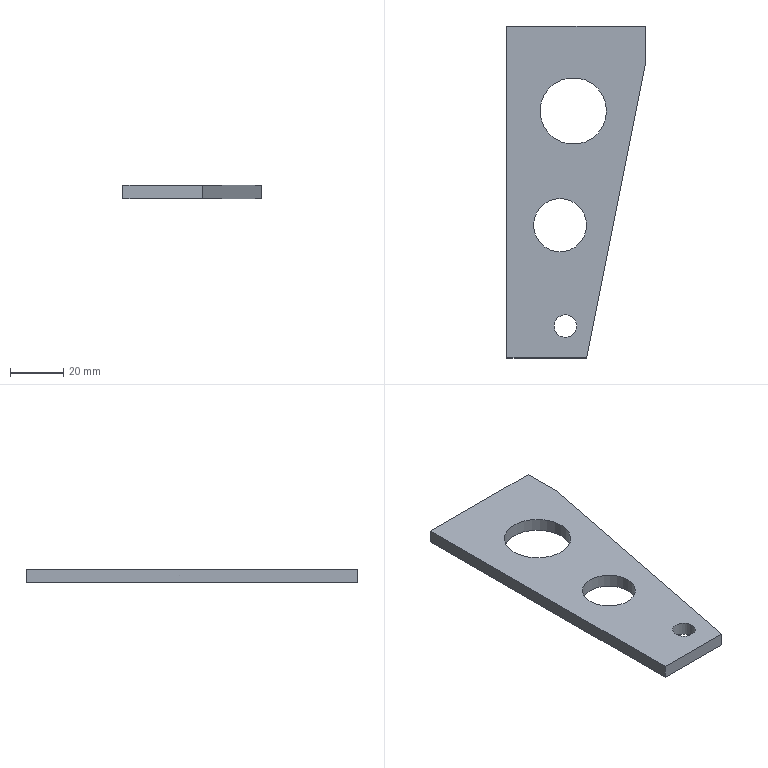Part | NX | features DATUM_CSYS 1, EXTRACT_DATUM_PLANE 1, EXTRUDE 1, SKETCH 1 | 1 solid | 10 faces | box 52 x 125 x 5 mm | volume 22141 mm3 | plane 7 | cylinder 3 | commonest cylinder face diameters 8.5 x1 20 x1 25 x1
STEP:
#1=CARTESIAN_POINT('',(-32.5,32.5,2.5));
#2=VERTEX_POINT('',#1);
#3=CARTESIAN_POINT('',(-32.5,-92.5,2.5));
#4=VERTEX_POINT('',#3);
#5=CARTESIAN_POINT('',(-32.5,32.5,2.5));
#6=DIRECTION('',(0.,-1.,0.));
#7=VECTOR('',#6,1000.);
#8=LINE('',#5,#7);
#9=EDGE_CURVE('',#2,#4,#8,.T.);
#10=ORIENTED_EDGE('',*,*,#9,.F.);
#11=CARTESIAN_POINT('',(-32.5,32.5,-2.5));
#12=VERTEX_POINT('',#11);
#13=CARTESIAN_POINT('',(-32.5,32.5,-2.5));
#14=DIRECTION('',(0.,0.,1.));
#15=VECTOR('',#14,1000.);
#16=LINE('',#13,#15);
#17=EDGE_CURVE('',#12,#2,#16,.T.);
#18=ORIENTED_EDGE('',*,*,#17,.F.);
#19=CARTESIAN_POINT('',(-32.5,-92.5,-2.5));
#20=VERTEX_POINT('',#19);
#21=CARTESIAN_POINT('',(-32.5,32.5,-2.5));
#22=DIRECTION('',(0.,-1.,0.));
#23=VECTOR('',#22,1000.);
#24=LINE('',#21,#23);
#25=EDGE_CURVE('',#12,#20,#24,.T.);
#26=ORIENTED_EDGE('',*,*,#25,.T.);
#27=CARTESIAN_POINT('',(-32.5,-92.5,-2.5));
#28=DIRECTION('',(0.,0.,1.));
#29=VECTOR('',#28,1000.);
#30=LINE('',#27,#29);
#31=EDGE_CURVE('',#20,#4,#30,.T.);
#32=ORIENTED_EDGE('',*,*,#31,.T.);
#33=EDGE_LOOP('',(#10,#18,#26,#32));
#34=FACE_BOUND('',#33,.T.);
#35=CARTESIAN_POINT('',(-32.5,32.5,-2.5));
#36=DIRECTION('',(-1.,0.,0.));
#37=DIRECTION('',(0.,0.,1.));
#38=AXIS2_PLACEMENT_3D('',#35,#36,#37);
#39=PLANE('',#38);
#40=ADVANCED_FACE('',(#34),#39,.T.);
#41=CARTESIAN_POINT('',(-2.5,-92.5,2.5));
#42=VERTEX_POINT('',#41);
#43=CARTESIAN_POINT('',(-32.5,-92.5,2.5));
#44=DIRECTION('',(1.,0.,0.));
#45=VECTOR('',#44,1000.);
#46=LINE('',#43,#45);
#47=EDGE_CURVE('',#4,#42,#46,.T.);
#48=ORIENTED_EDGE('',*,*,#47,.F.);
#49=ORIENTED_EDGE('',*,*,#31,.F.);
#50=CARTESIAN_POINT('',(-2.5,-92.5,-2.5));
#51=VERTEX_POINT('',#50);
#52=CARTESIAN_POINT('',(-32.5,-92.5,-2.5));
#53=DIRECTION('',(1.,0.,0.));
#54=VECTOR('',#53,1000.);
#55=LINE('',#52,#54);
#56=EDGE_CURVE('',#20,#51,#55,.T.);
#57=ORIENTED_EDGE('',*,*,#56,.T.);
#58=CARTESIAN_POINT('',(-2.5,-92.5,-2.5));
#59=DIRECTION('',(0.,0.,1.));
#60=VECTOR('',#59,1000.);
#61=LINE('',#58,#60);
#62=EDGE_CURVE('',#51,#42,#61,.T.);
#63=ORIENTED_EDGE('',*,*,#62,.T.);
#64=EDGE_LOOP('',(#48,#49,#57,#63));
#65=FACE_BOUND('',#64,.T.);
#66=CARTESIAN_POINT('',(-32.5,-92.5,-2.5));
#67=DIRECTION('',(0.,-1.,0.));
#68=DIRECTION('',(0.,0.,-1.));
#69=AXIS2_PLACEMENT_3D('',#66,#67,#68);
#70=PLANE('',#69);
#71=ADVANCED_FACE('',(#65),#70,.T.);
#72=CARTESIAN_POINT('',(19.5,17.5,2.5));
#73=VERTEX_POINT('',#72);
#74=CARTESIAN_POINT('',(-2.5,-92.5,2.5));
#75=DIRECTION('',(0.1961,0.9806,0.));
#76=VECTOR('',#75,1000.);
#77=LINE('',#74,#76);
#78=EDGE_CURVE('',#42,#73,#77,.T.);
#79=ORIENTED_EDGE('',*,*,#78,.F.);
#80=ORIENTED_EDGE('',*,*,#62,.F.);
#81=CARTESIAN_POINT('',(19.5,17.5,-2.5));
#82=VERTEX_POINT('',#81);
#83=CARTESIAN_POINT('',(-2.5,-92.5,-2.5));
#84=DIRECTION('',(0.1961,0.9806,0.));
#85=VECTOR('',#84,1000.);
#86=LINE('',#83,#85);
#87=EDGE_CURVE('',#51,#82,#86,.T.);
#88=ORIENTED_EDGE('',*,*,#87,.T.);
#89=CARTESIAN_POINT('',(19.5,17.5,-2.5));
#90=DIRECTION('',(0.,0.,1.));
#91=VECTOR('',#90,1000.);
#92=LINE('',#89,#91);
#93=EDGE_CURVE('',#82,#73,#92,.T.);
#94=ORIENTED_EDGE('',*,*,#93,.T.);
#95=EDGE_LOOP('',(#79,#80,#88,#94));
#96=FACE_BOUND('',#95,.T.);
#97=CARTESIAN_POINT('',(-2.5,-92.5,-2.5));
#98=DIRECTION('',(0.9806,-0.1961,0.));
#99=DIRECTION('',(0.1961,0.9806,0.));
#100=AXIS2_PLACEMENT_3D('',#97,#98,#99);
#101=PLANE('',#100);
#102=ADVANCED_FACE('',(#96),#101,.T.);
#103=CARTESIAN_POINT('',(19.5,32.5,2.5));
#104=VERTEX_POINT('',#103);
#105=CARTESIAN_POINT('',(19.5,17.5,2.5));
#106=DIRECTION('',(0.,1.,0.));
#107=VECTOR('',#106,1000.);
#108=LINE('',#105,#107);
#109=EDGE_CURVE('',#73,#104,#108,.T.);
#110=ORIENTED_EDGE('',*,*,#109,.F.);
#111=ORIENTED_EDGE('',*,*,#93,.F.);
#112=CARTESIAN_POINT('',(19.5,32.5,-2.5));
#113=VERTEX_POINT('',#112);
#114=CARTESIAN_POINT('',(19.5,17.5,-2.5));
#115=DIRECTION('',(0.,1.,0.));
#116=VECTOR('',#115,1000.);
#117=LINE('',#114,#116);
#118=EDGE_CURVE('',#82,#113,#117,.T.);
#119=ORIENTED_EDGE('',*,*,#118,.T.);
#120=CARTESIAN_POINT('',(19.5,32.5,-2.5));
#121=DIRECTION('',(0.,0.,1.));
#122=VECTOR('',#121,1000.);
#123=LINE('',#120,#122);
#124=EDGE_CURVE('',#113,#104,#123,.T.);
#125=ORIENTED_EDGE('',*,*,#124,.T.);
#126=EDGE_LOOP('',(#110,#111,#119,#125));
#127=FACE_BOUND('',#126,.T.);
#128=CARTESIAN_POINT('',(19.5,17.5,-2.5));
#129=DIRECTION('',(1.,0.,0.));
#130=DIRECTION('',(0.,0.,-1.));
#131=AXIS2_PLACEMENT_3D('',#128,#129,#130);
#132=PLANE('',#131);
#133=ADVANCED_FACE('',(#127),#132,.T.);
#134=CARTESIAN_POINT('',(-20.,0.5,2.5));
#135=VERTEX_POINT('',#134);
#136=CARTESIAN_POINT('',(-7.5,0.5,2.5));
#137=DIRECTION('',(0.,0.,-1.));
#138=DIRECTION('',(-1.,0.,0.));
#139=AXIS2_PLACEMENT_3D('',#136,#137,#138);
#140=CIRCLE('',#139,12.5);
#141=EDGE_CURVE('',#135,#135,#140,.T.);
#142=ORIENTED_EDGE('',*,*,#141,.F.);
#143=EDGE_LOOP('',(#142));
#144=FACE_BOUND('',#143,.T.);
#145=CARTESIAN_POINT('',(5.,0.5,-2.5));
#146=VERTEX_POINT('',#145);
#147=CARTESIAN_POINT('',(-7.5,0.5,-2.5));
#148=DIRECTION('',(0.,0.,-1.));
#149=DIRECTION('',(1.,0.,0.));
#150=AXIS2_PLACEMENT_3D('',#147,#148,#149);
#151=CIRCLE('',#150,12.5);
#152=EDGE_CURVE('',#146,#146,#151,.T.);
#153=ORIENTED_EDGE('',*,*,#152,.T.);
#154=EDGE_LOOP('',(#153));
#155=FACE_BOUND('',#154,.T.);
#156=CARTESIAN_POINT('',(-7.5,0.5,-2.5));
#157=DIRECTION('',(0.,0.,1.));
#158=DIRECTION('',(1.,0.,0.));
#159=AXIS2_PLACEMENT_3D('',#156,#157,#158);
#160=CYLINDRICAL_SURFACE('',#159,12.5);
#161=ADVANCED_FACE('',(#144,#155),#160,.F.);
#162=CARTESIAN_POINT('',(-22.5,-42.5,2.5));
#163=VERTEX_POINT('',#162);
#164=CARTESIAN_POINT('',(-12.5,-42.5,2.5));
#165=DIRECTION('',(0.,0.,-1.));
#166=DIRECTION('',(-1.,0.,0.));
#167=AXIS2_PLACEMENT_3D('',#164,#165,#166);
#168=CIRCLE('',#167,10.);
#169=EDGE_CURVE('',#163,#163,#168,.T.);
#170=ORIENTED_EDGE('',*,*,#169,.F.);
#171=EDGE_LOOP('',(#170));
#172=FACE_BOUND('',#171,.T.);
#173=CARTESIAN_POINT('',(-2.5,-42.5,-2.5));
#174=VERTEX_POINT('',#173);
#175=CARTESIAN_POINT('',(-12.5,-42.5,-2.5));
#176=DIRECTION('',(0.,0.,-1.));
#177=DIRECTION('',(1.,0.,0.));
#178=AXIS2_PLACEMENT_3D('',#175,#176,#177);
#179=CIRCLE('',#178,10.);
#180=EDGE_CURVE('',#174,#174,#179,.T.);
#181=ORIENTED_EDGE('',*,*,#180,.T.);
#182=EDGE_LOOP('',(#181));
#183=FACE_BOUND('',#182,.T.);
#184=CARTESIAN_POINT('',(-12.5,-42.5,-2.5));
#185=DIRECTION('',(0.,0.,1.));
#186=DIRECTION('',(1.,0.,0.));
#187=AXIS2_PLACEMENT_3D('',#184,#185,#186);
#188=CYLINDRICAL_SURFACE('',#187,10.);
#189=ADVANCED_FACE('',(#172,#183),#188,.F.);
#190=CARTESIAN_POINT('',(19.5,32.5,2.5));
#191=DIRECTION('',(-1.,0.,0.));
#192=VECTOR('',#191,1000.);
#193=LINE('',#190,#192);
#194=EDGE_CURVE('',#104,#2,#193,.T.);
#195=ORIENTED_EDGE('',*,*,#194,.F.);
#196=ORIENTED_EDGE('',*,*,#124,.F.);
#197=CARTESIAN_POINT('',(19.5,32.5,-2.5));
#198=DIRECTION('',(-1.,0.,0.));
#199=VECTOR('',#198,1000.);
#200=LINE('',#197,#199);
#201=EDGE_CURVE('',#113,#12,#200,.T.);
#202=ORIENTED_EDGE('',*,*,#201,.T.);
#203=ORIENTED_EDGE('',*,*,#17,.T.);
#204=EDGE_LOOP('',(#195,#196,#202,#203));
#205=FACE_BOUND('',#204,.T.);
#206=CARTESIAN_POINT('',(19.5,32.5,-2.5));
#207=DIRECTION('',(0.,1.,0.));
#208=DIRECTION('',(0.,0.,1.));
#209=AXIS2_PLACEMENT_3D('',#206,#207,#208);
#210=PLANE('',#209);
#211=ADVANCED_FACE('',(#205),#210,.T.);
#212=CARTESIAN_POINT('',(-14.75,-80.5,2.5));
#213=VERTEX_POINT('',#212);
#214=CARTESIAN_POINT('',(-10.5,-80.5,2.5));
#215=DIRECTION('',(0.,0.,-1.));
#216=DIRECTION('',(-1.,0.,0.));
#217=AXIS2_PLACEMENT_3D('',#214,#215,#216);
#218=CIRCLE('',#217,4.25);
#219=EDGE_CURVE('',#213,#213,#218,.T.);
#220=ORIENTED_EDGE('',*,*,#219,.F.);
#221=EDGE_LOOP('',(#220));
#222=FACE_BOUND('',#221,.T.);
#223=CARTESIAN_POINT('',(-6.25,-80.5,-2.5));
#224=VERTEX_POINT('',#223);
#225=CARTESIAN_POINT('',(-10.5,-80.5,-2.5));
#226=DIRECTION('',(0.,0.,-1.));
#227=DIRECTION('',(1.,0.,0.));
#228=AXIS2_PLACEMENT_3D('',#225,#226,#227);
#229=CIRCLE('',#228,4.25);
#230=EDGE_CURVE('',#224,#224,#229,.T.);
#231=ORIENTED_EDGE('',*,*,#230,.T.);
#232=EDGE_LOOP('',(#231));
#233=FACE_BOUND('',#232,.T.);
#234=CARTESIAN_POINT('',(-10.5,-80.5,-2.5));
#235=DIRECTION('',(0.,0.,1.));
#236=DIRECTION('',(1.,0.,0.));
#237=AXIS2_PLACEMENT_3D('',#234,#235,#236);
#238=CYLINDRICAL_SURFACE('',#237,4.25);
#239=ADVANCED_FACE('',(#222,#233),#238,.F.);
#240=ORIENTED_EDGE('',*,*,#25,.F.);
#241=ORIENTED_EDGE('',*,*,#201,.F.);
#242=ORIENTED_EDGE('',*,*,#118,.F.);
#243=ORIENTED_EDGE('',*,*,#87,.F.);
#244=ORIENTED_EDGE('',*,*,#56,.F.);
#245=EDGE_LOOP('',(#240,#241,#242,#243,#244));
#246=FACE_BOUND('',#245,.T.);
#247=ORIENTED_EDGE('',*,*,#180,.F.);
#248=EDGE_LOOP('',(#247));
#249=FACE_BOUND('',#248,.T.);
#250=ORIENTED_EDGE('',*,*,#152,.F.);
#251=EDGE_LOOP('',(#250));
#252=FACE_BOUND('',#251,.T.);
#253=ORIENTED_EDGE('',*,*,#230,.F.);
#254=EDGE_LOOP('',(#253));
#255=FACE_BOUND('',#254,.T.);
#256=CARTESIAN_POINT('',(-12.5,-42.5,-2.5));
#257=DIRECTION('',(0.,0.,-1.));
#258=DIRECTION('',(-1.,0.,0.));
#259=AXIS2_PLACEMENT_3D('',#256,#257,#258);
#260=PLANE('',#259);
#261=ADVANCED_FACE('',(#246,#249,#252,#255),#260,.T.);
#262=ORIENTED_EDGE('',*,*,#9,.T.);
#263=ORIENTED_EDGE('',*,*,#47,.T.);
#264=ORIENTED_EDGE('',*,*,#78,.T.);
#265=ORIENTED_EDGE('',*,*,#109,.T.);
#266=ORIENTED_EDGE('',*,*,#194,.T.);
#267=EDGE_LOOP('',(#262,#263,#264,#265,#266));
#268=FACE_BOUND('',#267,.T.);
#269=ORIENTED_EDGE('',*,*,#169,.T.);
#270=EDGE_LOOP('',(#269));
#271=FACE_BOUND('',#270,.T.);
#272=ORIENTED_EDGE('',*,*,#141,.T.);
#273=EDGE_LOOP('',(#272));
#274=FACE_BOUND('',#273,.T.);
#275=ORIENTED_EDGE('',*,*,#219,.T.);
#276=EDGE_LOOP('',(#275));
#277=FACE_BOUND('',#276,.T.);
#278=CARTESIAN_POINT('',(-12.5,-42.5,2.5));
#279=DIRECTION('',(0.,0.,-1.));
#280=DIRECTION('',(-1.,0.,0.));
#281=AXIS2_PLACEMENT_3D('',#278,#279,#280);
#282=PLANE('',#281);
#283=ADVANCED_FACE('',(#268,#271,#274,#277),#282,.F.);
#284=CLOSED_SHELL('',(#40,#71,#102,#133,#161,#189,#211,#239,#261,#283));
#285=MANIFOLD_SOLID_BREP('',#284);
#286=(LENGTH_UNIT()NAMED_UNIT(*)SI_UNIT(.MILLI.,.METRE.));
#287=UNCERTAINTY_MEASURE_WITH_UNIT(LENGTH_MEASURE(0.00001),#286,'','');
#288=(NAMED_UNIT(*)PLANE_ANGLE_UNIT()SI_UNIT($,.RADIAN.));
#289=(NAMED_UNIT(*)SI_UNIT($,.STERADIAN.)SOLID_ANGLE_UNIT());
#290=(GEOMETRIC_REPRESENTATION_CONTEXT(3)GLOBAL_UNCERTAINTY_ASSIGNED_CONTEXT((#287))GLOBAL_UNIT_ASSIGNED_CONTEXT((#286,#288,#289))REPRESENTATION_CONTEXT('',''));
#291=ADVANCED_BREP_SHAPE_REPRESENTATION('',(#285),#290);